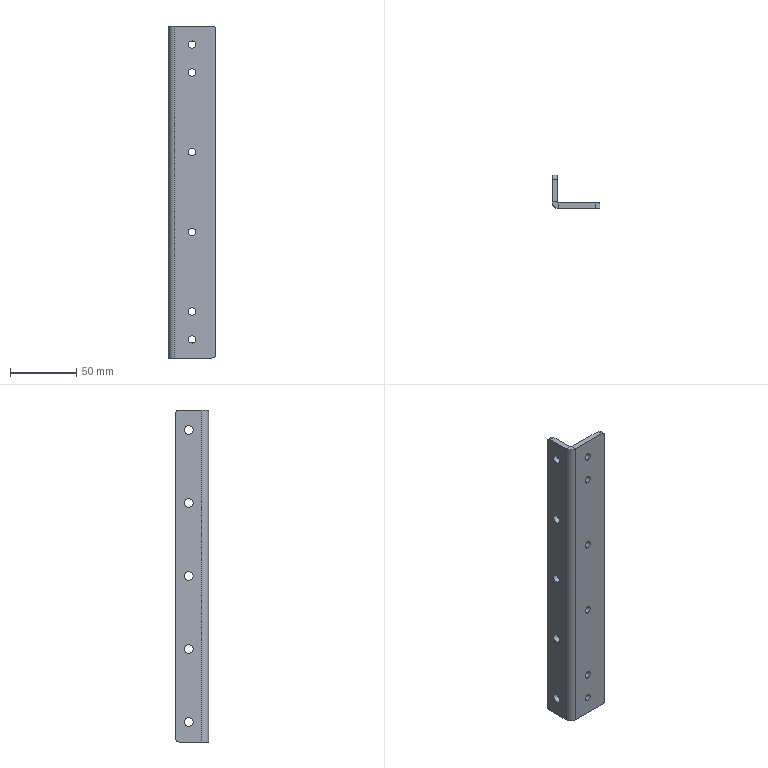Part | STEP file | Part 1 cang dai | 1 solid | 40 faces | box 36 x 25 x 250 mm | volume 54427 mm3 | cylinder 28 | plane 12 | commonest cylinder face diameters 5.5 x12 6.6 x10 6 x4 2 x1 10 x1
STEP:
#1=CARTESIAN_POINT('',(0.,15.,113.3));
#2=VERTEX_POINT('',#1);
#3=CARTESIAN_POINT('',(0.,15.,106.7));
#4=VERTEX_POINT('',#3);
#5=CARTESIAN_POINT('',(0.,15.,110.));
#6=DIRECTION('',(1.,0.,0.));
#7=DIRECTION('',(0.,0.,-1.));
#8=AXIS2_PLACEMENT_3D('',#5,#6,#7);
#9=CIRCLE('',#8,3.3);
#10=EDGE_CURVE('',#2,#4,#9,.T.);
#11=ORIENTED_EDGE('',*,*,#10,.F.);
#12=CARTESIAN_POINT('',(4.,15.,113.3));
#13=VERTEX_POINT('',#12);
#14=CARTESIAN_POINT('',(4.,15.,113.3));
#15=DIRECTION('',(1.,0.,0.));
#16=VECTOR('',#15,1000.);
#17=LINE('',#14,#16);
#18=EDGE_CURVE('',#2,#13,#17,.T.);
#19=ORIENTED_EDGE('',*,*,#18,.T.);
#20=CARTESIAN_POINT('',(4.,15.,106.7));
#21=VERTEX_POINT('',#20);
#22=CARTESIAN_POINT('',(4.,15.,110.));
#23=DIRECTION('',(1.,0.,0.));
#24=DIRECTION('',(0.,0.,-1.));
#25=AXIS2_PLACEMENT_3D('',#22,#23,#24);
#26=CIRCLE('',#25,3.3);
#27=EDGE_CURVE('',#13,#21,#26,.T.);
#28=ORIENTED_EDGE('',*,*,#27,.T.);
#29=CARTESIAN_POINT('',(4.,15.,106.7));
#30=DIRECTION('',(1.,0.,0.));
#31=VECTOR('',#30,1000.);
#32=LINE('',#29,#31);
#33=EDGE_CURVE('',#4,#21,#32,.T.);
#34=ORIENTED_EDGE('',*,*,#33,.F.);
#35=EDGE_LOOP('',(#11,#19,#28,#34));
#36=FACE_OUTER_BOUND('',#35,.T.);
#37=CARTESIAN_POINT('',(4.,15.,110.));
#38=DIRECTION('',(1.,0.,0.));
#39=DIRECTION('',(0.,0.,-1.));
#40=AXIS2_PLACEMENT_3D('',#37,#38,#39);
#41=CYLINDRICAL_SURFACE('',#40,3.3);
#42=ADVANCED_FACE('',(#36),#41,.F.);
#43=CARTESIAN_POINT('',(0.,15.,58.3));
#44=VERTEX_POINT('',#43);
#45=CARTESIAN_POINT('',(0.,15.,51.7));
#46=VERTEX_POINT('',#45);
#47=CARTESIAN_POINT('',(0.,15.,55.));
#48=DIRECTION('',(1.,0.,0.));
#49=DIRECTION('',(0.,0.,-1.));
#50=AXIS2_PLACEMENT_3D('',#47,#48,#49);
#51=CIRCLE('',#50,3.3);
#52=EDGE_CURVE('',#44,#46,#51,.T.);
#53=ORIENTED_EDGE('',*,*,#52,.F.);
#54=CARTESIAN_POINT('',(4.,15.,58.3));
#55=VERTEX_POINT('',#54);
#56=CARTESIAN_POINT('',(4.,15.,58.3));
#57=DIRECTION('',(1.,0.,0.));
#58=VECTOR('',#57,1000.);
#59=LINE('',#56,#58);
#60=EDGE_CURVE('',#44,#55,#59,.T.);
#61=ORIENTED_EDGE('',*,*,#60,.T.);
#62=CARTESIAN_POINT('',(4.,15.,51.7));
#63=VERTEX_POINT('',#62);
#64=CARTESIAN_POINT('',(4.,15.,55.));
#65=DIRECTION('',(1.,0.,0.));
#66=DIRECTION('',(0.,0.,-1.));
#67=AXIS2_PLACEMENT_3D('',#64,#65,#66);
#68=CIRCLE('',#67,3.3);
#69=EDGE_CURVE('',#55,#63,#68,.T.);
#70=ORIENTED_EDGE('',*,*,#69,.T.);
#71=CARTESIAN_POINT('',(4.,15.,51.7));
#72=DIRECTION('',(1.,0.,0.));
#73=VECTOR('',#72,1000.);
#74=LINE('',#71,#73);
#75=EDGE_CURVE('',#46,#63,#74,.T.);
#76=ORIENTED_EDGE('',*,*,#75,.F.);
#77=EDGE_LOOP('',(#53,#61,#70,#76));
#78=FACE_OUTER_BOUND('',#77,.T.);
#79=CARTESIAN_POINT('',(4.,15.,55.));
#80=DIRECTION('',(1.,0.,0.));
#81=DIRECTION('',(0.,0.,-1.));
#82=AXIS2_PLACEMENT_3D('',#79,#80,#81);
#83=CYLINDRICAL_SURFACE('',#82,3.3);
#84=ADVANCED_FACE('',(#78),#83,.F.);
#85=CARTESIAN_POINT('',(0.,15.,3.3));
#86=VERTEX_POINT('',#85);
#87=CARTESIAN_POINT('',(0.,15.,-3.3));
#88=VERTEX_POINT('',#87);
#89=CARTESIAN_POINT('',(0.,15.,0.));
#90=DIRECTION('',(1.,0.,0.));
#91=DIRECTION('',(0.,0.,-1.));
#92=AXIS2_PLACEMENT_3D('',#89,#90,#91);
#93=CIRCLE('',#92,3.3);
#94=EDGE_CURVE('',#86,#88,#93,.T.);
#95=ORIENTED_EDGE('',*,*,#94,.F.);
#96=CARTESIAN_POINT('',(4.,15.,3.3));
#97=VERTEX_POINT('',#96);
#98=CARTESIAN_POINT('',(4.,15.,3.3));
#99=DIRECTION('',(1.,0.,0.));
#100=VECTOR('',#99,1000.);
#101=LINE('',#98,#100);
#102=EDGE_CURVE('',#86,#97,#101,.T.);
#103=ORIENTED_EDGE('',*,*,#102,.T.);
#104=CARTESIAN_POINT('',(4.,15.,-3.3));
#105=VERTEX_POINT('',#104);
#106=CARTESIAN_POINT('',(4.,15.,0.));
#107=DIRECTION('',(1.,0.,0.));
#108=DIRECTION('',(0.,0.,-1.));
#109=AXIS2_PLACEMENT_3D('',#106,#107,#108);
#110=CIRCLE('',#109,3.3);
#111=EDGE_CURVE('',#97,#105,#110,.T.);
#112=ORIENTED_EDGE('',*,*,#111,.T.);
#113=CARTESIAN_POINT('',(4.,15.,-3.3));
#114=DIRECTION('',(1.,0.,0.));
#115=VECTOR('',#114,1000.);
#116=LINE('',#113,#115);
#117=EDGE_CURVE('',#88,#105,#116,.T.);
#118=ORIENTED_EDGE('',*,*,#117,.F.);
#119=EDGE_LOOP('',(#95,#103,#112,#118));
#120=FACE_OUTER_BOUND('',#119,.T.);
#121=CARTESIAN_POINT('',(4.,15.,0.));
#122=DIRECTION('',(1.,0.,0.));
#123=DIRECTION('',(0.,0.,-1.));
#124=AXIS2_PLACEMENT_3D('',#121,#122,#123);
#125=CYLINDRICAL_SURFACE('',#124,3.3);
#126=ADVANCED_FACE('',(#120),#125,.F.);
#127=CARTESIAN_POINT('',(0.,15.,-51.7));
#128=VERTEX_POINT('',#127);
#129=CARTESIAN_POINT('',(0.,15.,-58.3));
#130=VERTEX_POINT('',#129);
#131=CARTESIAN_POINT('',(0.,15.,-55.));
#132=DIRECTION('',(1.,0.,0.));
#133=DIRECTION('',(0.,0.,-1.));
#134=AXIS2_PLACEMENT_3D('',#131,#132,#133);
#135=CIRCLE('',#134,3.3);
#136=EDGE_CURVE('',#128,#130,#135,.T.);
#137=ORIENTED_EDGE('',*,*,#136,.F.);
#138=CARTESIAN_POINT('',(4.,15.,-51.7));
#139=VERTEX_POINT('',#138);
#140=CARTESIAN_POINT('',(4.,15.,-51.7));
#141=DIRECTION('',(1.,0.,0.));
#142=VECTOR('',#141,1000.);
#143=LINE('',#140,#142);
#144=EDGE_CURVE('',#128,#139,#143,.T.);
#145=ORIENTED_EDGE('',*,*,#144,.T.);
#146=CARTESIAN_POINT('',(4.,15.,-58.3));
#147=VERTEX_POINT('',#146);
#148=CARTESIAN_POINT('',(4.,15.,-55.));
#149=DIRECTION('',(1.,0.,0.));
#150=DIRECTION('',(0.,0.,-1.));
#151=AXIS2_PLACEMENT_3D('',#148,#149,#150);
#152=CIRCLE('',#151,3.3);
#153=EDGE_CURVE('',#139,#147,#152,.T.);
#154=ORIENTED_EDGE('',*,*,#153,.T.);
#155=CARTESIAN_POINT('',(4.,15.,-58.3));
#156=DIRECTION('',(1.,0.,0.));
#157=VECTOR('',#156,1000.);
#158=LINE('',#155,#157);
#159=EDGE_CURVE('',#130,#147,#158,.T.);
#160=ORIENTED_EDGE('',*,*,#159,.F.);
#161=EDGE_LOOP('',(#137,#145,#154,#160));
#162=FACE_OUTER_BOUND('',#161,.T.);
#163=CARTESIAN_POINT('',(4.,15.,-55.));
#164=DIRECTION('',(1.,0.,0.));
#165=DIRECTION('',(0.,0.,-1.));
#166=AXIS2_PLACEMENT_3D('',#163,#164,#165);
#167=CYLINDRICAL_SURFACE('',#166,3.3);
#168=ADVANCED_FACE('',(#162),#167,.F.);
#169=CARTESIAN_POINT('',(0.,15.,-106.7));
#170=VERTEX_POINT('',#169);
#171=CARTESIAN_POINT('',(0.,15.,-113.3));
#172=VERTEX_POINT('',#171);
#173=CARTESIAN_POINT('',(0.,15.,-110.));
#174=DIRECTION('',(1.,0.,0.));
#175=DIRECTION('',(0.,0.,-1.));
#176=AXIS2_PLACEMENT_3D('',#173,#174,#175);
#177=CIRCLE('',#176,3.3);
#178=EDGE_CURVE('',#170,#172,#177,.T.);
#179=ORIENTED_EDGE('',*,*,#178,.F.);
#180=CARTESIAN_POINT('',(4.,15.,-106.7));
#181=VERTEX_POINT('',#180);
#182=CARTESIAN_POINT('',(4.,15.,-106.7));
#183=DIRECTION('',(1.,0.,0.));
#184=VECTOR('',#183,1000.);
#185=LINE('',#182,#184);
#186=EDGE_CURVE('',#170,#181,#185,.T.);
#187=ORIENTED_EDGE('',*,*,#186,.T.);
#188=CARTESIAN_POINT('',(4.,15.,-113.3));
#189=VERTEX_POINT('',#188);
#190=CARTESIAN_POINT('',(4.,15.,-110.));
#191=DIRECTION('',(1.,0.,0.));
#192=DIRECTION('',(0.,0.,-1.));
#193=AXIS2_PLACEMENT_3D('',#190,#191,#192);
#194=CIRCLE('',#193,3.3);
#195=EDGE_CURVE('',#181,#189,#194,.T.);
#196=ORIENTED_EDGE('',*,*,#195,.T.);
#197=CARTESIAN_POINT('',(4.,15.,-113.3));
#198=DIRECTION('',(1.,0.,0.));
#199=VECTOR('',#198,1000.);
#200=LINE('',#197,#199);
#201=EDGE_CURVE('',#172,#189,#200,.T.);
#202=ORIENTED_EDGE('',*,*,#201,.F.);
#203=EDGE_LOOP('',(#179,#187,#196,#202));
#204=FACE_OUTER_BOUND('',#203,.T.);
#205=CARTESIAN_POINT('',(4.,15.,-110.));
#206=DIRECTION('',(1.,0.,0.));
#207=DIRECTION('',(0.,0.,-1.));
#208=AXIS2_PLACEMENT_3D('',#205,#206,#207);
#209=CYLINDRICAL_SURFACE('',#208,3.3);
#210=ADVANCED_FACE('',(#204),#209,.F.);
#211=CARTESIAN_POINT('',(18.,0.,108.25));
#212=VERTEX_POINT('',#211);
#213=CARTESIAN_POINT('',(18.,0.,113.75));
#214=VERTEX_POINT('',#213);
#215=CARTESIAN_POINT('',(18.,0.,111.));
#216=DIRECTION('',(0.,1.,0.));
#217=DIRECTION('',(0.,0.,1.));
#218=AXIS2_PLACEMENT_3D('',#215,#216,#217);
#219=CIRCLE('',#218,2.75);
#220=EDGE_CURVE('',#212,#214,#219,.T.);
#221=ORIENTED_EDGE('',*,*,#220,.F.);
#222=CARTESIAN_POINT('',(18.,4.,108.25));
#223=VERTEX_POINT('',#222);
#224=CARTESIAN_POINT('',(18.,4.,108.25));
#225=DIRECTION('',(0.,1.,0.));
#226=VECTOR('',#225,1000.);
#227=LINE('',#224,#226);
#228=EDGE_CURVE('',#212,#223,#227,.T.);
#229=ORIENTED_EDGE('',*,*,#228,.T.);
#230=CARTESIAN_POINT('',(18.,4.,113.75));
#231=VERTEX_POINT('',#230);
#232=CARTESIAN_POINT('',(18.,4.,111.));
#233=DIRECTION('',(0.,1.,0.));
#234=DIRECTION('',(0.,0.,1.));
#235=AXIS2_PLACEMENT_3D('',#232,#233,#234);
#236=CIRCLE('',#235,2.75);
#237=EDGE_CURVE('',#223,#231,#236,.T.);
#238=ORIENTED_EDGE('',*,*,#237,.T.);
#239=CARTESIAN_POINT('',(18.,4.,113.75));
#240=DIRECTION('',(0.,1.,0.));
#241=VECTOR('',#240,1000.);
#242=LINE('',#239,#241);
#243=EDGE_CURVE('',#214,#231,#242,.T.);
#244=ORIENTED_EDGE('',*,*,#243,.F.);
#245=EDGE_LOOP('',(#221,#229,#238,#244));
#246=FACE_OUTER_BOUND('',#245,.T.);
#247=CARTESIAN_POINT('',(18.,4.,111.));
#248=DIRECTION('',(0.,1.,0.));
#249=DIRECTION('',(0.,0.,1.));
#250=AXIS2_PLACEMENT_3D('',#247,#248,#249);
#251=CYLINDRICAL_SURFACE('',#250,2.75);
#252=ADVANCED_FACE('',(#246),#251,.F.);
#253=CARTESIAN_POINT('',(18.,0.,-113.75));
#254=VERTEX_POINT('',#253);
#255=CARTESIAN_POINT('',(18.,0.,-108.25));
#256=VERTEX_POINT('',#255);
#257=CARTESIAN_POINT('',(18.,0.,-111.));
#258=DIRECTION('',(0.,1.,0.));
#259=DIRECTION('',(0.,0.,1.));
#260=AXIS2_PLACEMENT_3D('',#257,#258,#259);
#261=CIRCLE('',#260,2.75);
#262=EDGE_CURVE('',#254,#256,#261,.T.);
#263=ORIENTED_EDGE('',*,*,#262,.F.);
#264=CARTESIAN_POINT('',(18.,4.,-113.75));
#265=VERTEX_POINT('',#264);
#266=CARTESIAN_POINT('',(18.,4.,-113.75));
#267=DIRECTION('',(0.,1.,0.));
#268=VECTOR('',#267,1000.);
#269=LINE('',#266,#268);
#270=EDGE_CURVE('',#254,#265,#269,.T.);
#271=ORIENTED_EDGE('',*,*,#270,.T.);
#272=CARTESIAN_POINT('',(18.,4.,-108.25));
#273=VERTEX_POINT('',#272);
#274=CARTESIAN_POINT('',(18.,4.,-111.));
#275=DIRECTION('',(0.,1.,0.));
#276=DIRECTION('',(0.,0.,1.));
#277=AXIS2_PLACEMENT_3D('',#274,#275,#276);
#278=CIRCLE('',#277,2.75);
#279=EDGE_CURVE('',#265,#273,#278,.T.);
#280=ORIENTED_EDGE('',*,*,#279,.T.);
#281=CARTESIAN_POINT('',(18.,4.,-108.25));
#282=DIRECTION('',(0.,1.,0.));
#283=VECTOR('',#282,1000.);
#284=LINE('',#281,#283);
#285=EDGE_CURVE('',#256,#273,#284,.T.);
#286=ORIENTED_EDGE('',*,*,#285,.F.);
#287=EDGE_LOOP('',(#263,#271,#280,#286));
#288=FACE_OUTER_BOUND('',#287,.T.);
#289=CARTESIAN_POINT('',(18.,4.,-111.));
#290=DIRECTION('',(0.,1.,0.));
#291=DIRECTION('',(0.,0.,1.));
#292=AXIS2_PLACEMENT_3D('',#289,#290,#291);
#293=CYLINDRICAL_SURFACE('',#292,2.75);
#294=ADVANCED_FACE('',(#288),#293,.F.);
#295=CARTESIAN_POINT('',(18.,0.,-92.75));
#296=VERTEX_POINT('',#295);
#297=CARTESIAN_POINT('',(18.,0.,-87.25));
#298=VERTEX_POINT('',#297);
#299=CARTESIAN_POINT('',(18.,0.,-90.));
#300=DIRECTION('',(0.,1.,0.));
#301=DIRECTION('',(0.,0.,1.));
#302=AXIS2_PLACEMENT_3D('',#299,#300,#301);
#303=CIRCLE('',#302,2.75);
#304=EDGE_CURVE('',#296,#298,#303,.T.);
#305=ORIENTED_EDGE('',*,*,#304,.F.);
#306=CARTESIAN_POINT('',(18.,4.,-92.75));
#307=VERTEX_POINT('',#306);
#308=CARTESIAN_POINT('',(18.,4.,-92.75));
#309=DIRECTION('',(0.,1.,0.));
#310=VECTOR('',#309,1000.);
#311=LINE('',#308,#310);
#312=EDGE_CURVE('',#296,#307,#311,.T.);
#313=ORIENTED_EDGE('',*,*,#312,.T.);
#314=CARTESIAN_POINT('',(18.,4.,-87.25));
#315=VERTEX_POINT('',#314);
#316=CARTESIAN_POINT('',(18.,4.,-90.));
#317=DIRECTION('',(0.,1.,0.));
#318=DIRECTION('',(0.,0.,1.));
#319=AXIS2_PLACEMENT_3D('',#316,#317,#318);
#320=CIRCLE('',#319,2.75);
#321=EDGE_CURVE('',#307,#315,#320,.T.);
#322=ORIENTED_EDGE('',*,*,#321,.T.);
#323=CARTESIAN_POINT('',(18.,4.,-87.25));
#324=DIRECTION('',(0.,1.,0.));
#325=VECTOR('',#324,1000.);
#326=LINE('',#323,#325);
#327=EDGE_CURVE('',#298,#315,#326,.T.);
#328=ORIENTED_EDGE('',*,*,#327,.F.);
#329=EDGE_LOOP('',(#305,#313,#322,#328));
#330=FACE_OUTER_BOUND('',#329,.T.);
#331=CARTESIAN_POINT('',(18.,4.,-90.));
#332=DIRECTION('',(0.,1.,0.));
#333=DIRECTION('',(0.,0.,1.));
#334=AXIS2_PLACEMENT_3D('',#331,#332,#333);
#335=CYLINDRICAL_SURFACE('',#334,2.75);
#336=ADVANCED_FACE('',(#330),#335,.F.);
#337=CARTESIAN_POINT('',(18.,0.,-32.75));
#338=VERTEX_POINT('',#337);
#339=CARTESIAN_POINT('',(18.,0.,-27.25));
#340=VERTEX_POINT('',#339);
#341=CARTESIAN_POINT('',(18.,0.,-30.));
#342=DIRECTION('',(0.,1.,0.));
#343=DIRECTION('',(0.,0.,1.));
#344=AXIS2_PLACEMENT_3D('',#341,#342,#343);
#345=CIRCLE('',#344,2.75);
#346=EDGE_CURVE('',#338,#340,#345,.T.);
#347=ORIENTED_EDGE('',*,*,#346,.F.);
#348=CARTESIAN_POINT('',(18.,4.,-32.75));
#349=VERTEX_POINT('',#348);
#350=CARTESIAN_POINT('',(18.,4.,-32.75));
#351=DIRECTION('',(0.,1.,0.));
#352=VECTOR('',#351,1000.);
#353=LINE('',#350,#352);
#354=EDGE_CURVE('',#338,#349,#353,.T.);
#355=ORIENTED_EDGE('',*,*,#354,.T.);
#356=CARTESIAN_POINT('',(18.,4.,-27.25));
#357=VERTEX_POINT('',#356);
#358=CARTESIAN_POINT('',(18.,4.,-30.));
#359=DIRECTION('',(0.,1.,0.));
#360=DIRECTION('',(0.,0.,1.));
#361=AXIS2_PLACEMENT_3D('',#358,#359,#360);
#362=CIRCLE('',#361,2.75);
#363=EDGE_CURVE('',#349,#357,#362,.T.);
#364=ORIENTED_EDGE('',*,*,#363,.T.);
#365=CARTESIAN_POINT('',(18.,4.,-27.25));
#366=DIRECTION('',(0.,1.,0.));
#367=VECTOR('',#366,1000.);
#368=LINE('',#365,#367);
#369=EDGE_CURVE('',#340,#357,#368,.T.);
#370=ORIENTED_EDGE('',*,*,#369,.F.);
#371=EDGE_LOOP('',(#347,#355,#364,#370));
#372=FACE_OUTER_BOUND('',#371,.T.);
#373=CARTESIAN_POINT('',(18.,4.,-30.));
#374=DIRECTION('',(0.,1.,0.));
#375=DIRECTION('',(0.,0.,1.));
#376=AXIS2_PLACEMENT_3D('',#373,#374,#375);
#377=CYLINDRICAL_SURFACE('',#376,2.75);
#378=ADVANCED_FACE('',(#372),#377,.F.);
#379=CARTESIAN_POINT('',(18.,0.,27.25));
#380=VERTEX_POINT('',#379);
#381=CARTESIAN_POINT('',(18.,0.,32.75));
#382=VERTEX_POINT('',#381);
#383=CARTESIAN_POINT('',(18.,0.,30.));
#384=DIRECTION('',(0.,1.,0.));
#385=DIRECTION('',(0.,0.,1.));
#386=AXIS2_PLACEMENT_3D('',#383,#384,#385);
#387=CIRCLE('',#386,2.75);
#388=EDGE_CURVE('',#380,#382,#387,.T.);
#389=ORIENTED_EDGE('',*,*,#388,.F.);
#390=CARTESIAN_POINT('',(18.,4.,27.25));
#391=VERTEX_POINT('',#390);
#392=CARTESIAN_POINT('',(18.,4.,27.25));
#393=DIRECTION('',(0.,1.,0.));
#394=VECTOR('',#393,1000.);
#395=LINE('',#392,#394);
#396=EDGE_CURVE('',#380,#391,#395,.T.);
#397=ORIENTED_EDGE('',*,*,#396,.T.);
#398=CARTESIAN_POINT('',(18.,4.,32.75));
#399=VERTEX_POINT('',#398);
#400=CARTESIAN_POINT('',(18.,4.,30.));
#401=DIRECTION('',(0.,1.,0.));
#402=DIRECTION('',(0.,0.,1.));
#403=AXIS2_PLACEMENT_3D('',#400,#401,#402);
#404=CIRCLE('',#403,2.75);
#405=EDGE_CURVE('',#391,#399,#404,.T.);
#406=ORIENTED_EDGE('',*,*,#405,.T.);
#407=CARTESIAN_POINT('',(18.,4.,32.75));
#408=DIRECTION('',(0.,1.,0.));
#409=VECTOR('',#408,1000.);
#410=LINE('',#407,#409);
#411=EDGE_CURVE('',#382,#399,#410,.T.);
#412=ORIENTED_EDGE('',*,*,#411,.F.);
#413=EDGE_LOOP('',(#389,#397,#406,#412));
#414=FACE_OUTER_BOUND('',#413,.T.);
#415=CARTESIAN_POINT('',(18.,4.,30.));
#416=DIRECTION('',(0.,1.,0.));
#417=DIRECTION('',(0.,0.,1.));
#418=AXIS2_PLACEMENT_3D('',#415,#416,#417);
#419=CYLINDRICAL_SURFACE('',#418,2.75);
#420=ADVANCED_FACE('',(#414),#419,.F.);
#421=CARTESIAN_POINT('',(18.,0.,87.25));
#422=VERTEX_POINT('',#421);
#423=CARTESIAN_POINT('',(18.,0.,92.75));
#424=VERTEX_POINT('',#423);
#425=CARTESIAN_POINT('',(18.,0.,90.));
#426=DIRECTION('',(0.,1.,0.));
#427=DIRECTION('',(0.,0.,1.));
#428=AXIS2_PLACEMENT_3D('',#425,#426,#427);
#429=CIRCLE('',#428,2.75);
#430=EDGE_CURVE('',#422,#424,#429,.T.);
#431=ORIENTED_EDGE('',*,*,#430,.F.);
#432=CARTESIAN_POINT('',(18.,4.,87.25));
#433=VERTEX_POINT('',#432);
#434=CARTESIAN_POINT('',(18.,4.,87.25));
#435=DIRECTION('',(0.,1.,0.));
#436=VECTOR('',#435,1000.);
#437=LINE('',#434,#436);
#438=EDGE_CURVE('',#422,#433,#437,.T.);
#439=ORIENTED_EDGE('',*,*,#438,.T.);
#440=CARTESIAN_POINT('',(18.,4.,92.75));
#441=VERTEX_POINT('',#440);
#442=CARTESIAN_POINT('',(18.,4.,90.));
#443=DIRECTION('',(0.,1.,0.));
#444=DIRECTION('',(0.,0.,1.));
#445=AXIS2_PLACEMENT_3D('',#442,#443,#444);
#446=CIRCLE('',#445,2.75);
#447=EDGE_CURVE('',#433,#441,#446,.T.);
#448=ORIENTED_EDGE('',*,*,#447,.T.);
#449=CARTESIAN_POINT('',(18.,4.,92.75));
#450=DIRECTION('',(0.,1.,0.));
#451=VECTOR('',#450,1000.);
#452=LINE('',#449,#451);
#453=EDGE_CURVE('',#424,#441,#452,.T.);
#454=ORIENTED_EDGE('',*,*,#453,.F.);
#455=EDGE_LOOP('',(#431,#439,#448,#454));
#456=FACE_OUTER_BOUND('',#455,.T.);
#457=CARTESIAN_POINT('',(18.,4.,90.));
#458=DIRECTION('',(0.,1.,0.));
#459=DIRECTION('',(0.,0.,1.));
#460=AXIS2_PLACEMENT_3D('',#457,#458,#459);
#461=CYLINDRICAL_SURFACE('',#460,2.75);
#462=ADVANCED_FACE('',(#456),#461,.F.);
#463=CARTESIAN_POINT('',(0.,5.,125.));
#464=VERTEX_POINT('',#463);
#465=CARTESIAN_POINT('',(4.,5.,125.));
#466=VERTEX_POINT('',#465);
#467=CARTESIAN_POINT('',(0.,5.,125.));
#468=DIRECTION('',(1.,0.,0.));
#469=VECTOR('',#468,1000.);
#470=LINE('',#467,#469);
#471=EDGE_CURVE('',#464,#466,#470,.T.);
#472=ORIENTED_EDGE('',*,*,#471,.F.);
#473=CARTESIAN_POINT('',(5.,0.,125.));
#474=VERTEX_POINT('',#473);
#475=CARTESIAN_POINT('',(5.,5.,125.));
#476=DIRECTION('',(0.,0.,1.));
#477=DIRECTION('',(-1.,0.,0.));
#478=AXIS2_PLACEMENT_3D('',#475,#476,#477);
#479=CIRCLE('',#478,5.);
#480=EDGE_CURVE('',#464,#474,#479,.T.);
#481=ORIENTED_EDGE('',*,*,#480,.T.);
#482=CARTESIAN_POINT('',(5.,4.,125.));
#483=VERTEX_POINT('',#482);
#484=CARTESIAN_POINT('',(5.,4.,125.));
#485=DIRECTION('',(0.,-1.,0.));
#486=VECTOR('',#485,1000.);
#487=LINE('',#484,#486);
#488=EDGE_CURVE('',#483,#474,#487,.T.);
#489=ORIENTED_EDGE('',*,*,#488,.F.);
#490=CARTESIAN_POINT('',(5.,5.,125.));
#491=DIRECTION('',(0.,0.,1.));
#492=DIRECTION('',(1.,0.,0.));
#493=AXIS2_PLACEMENT_3D('',#490,#491,#492);
#494=CIRCLE('',#493,1.);
#495=EDGE_CURVE('',#466,#483,#494,.T.);
#496=ORIENTED_EDGE('',*,*,#495,.F.);
#497=EDGE_LOOP('',(#472,#481,#489,#496));
#498=FACE_OUTER_BOUND('',#497,.T.);
#499=CARTESIAN_POINT('',(0.,5.,125.));
#500=DIRECTION('',(0.,0.,1.));
#501=DIRECTION('',(1.,0.,0.));
#502=AXIS2_PLACEMENT_3D('',#499,#500,#501);
#503=PLANE('',#502);
#504=ADVANCED_FACE('',(#498),#503,.T.);
#505=CARTESIAN_POINT('',(4.,22.,125.));
#506=VERTEX_POINT('',#505);
#507=CARTESIAN_POINT('',(4.,0.,125.));
#508=DIRECTION('',(0.,-1.,0.));
#509=VECTOR('',#508,1000.);
#510=LINE('',#507,#509);
#511=EDGE_CURVE('',#506,#466,#510,.T.);
#512=ORIENTED_EDGE('',*,*,#511,.F.);
#513=CARTESIAN_POINT('',(0.,22.,125.));
#514=VERTEX_POINT('',#513);
#515=CARTESIAN_POINT('',(5.,22.,125.));
#516=DIRECTION('',(-1.,0.,0.));
#517=VECTOR('',#516,1000.);
#518=LINE('',#515,#517);
#519=EDGE_CURVE('',#506,#514,#518,.T.);
#520=ORIENTED_EDGE('',*,*,#519,.T.);
#521=CARTESIAN_POINT('',(0.,0.,125.));
#522=DIRECTION('',(0.,-1.,0.));
#523=VECTOR('',#522,1000.);
#524=LINE('',#521,#523);
#525=EDGE_CURVE('',#514,#464,#524,.T.);
#526=ORIENTED_EDGE('',*,*,#525,.T.);
#527=ORIENTED_EDGE('',*,*,#471,.T.);
#528=EDGE_LOOP('',(#512,#520,#526,#527));
#529=FACE_OUTER_BOUND('',#528,.T.);
#530=CARTESIAN_POINT('',(5.,4.,125.));
#531=DIRECTION('',(0.,0.,1.));
#532=DIRECTION('',(1.,0.,0.));
#533=AXIS2_PLACEMENT_3D('',#530,#531,#532);
#534=PLANE('',#533);
#535=ADVANCED_FACE('',(#529),#534,.T.);
#536=CARTESIAN_POINT('',(5.,0.,-125.));
#537=VERTEX_POINT('',#536);
#538=CARTESIAN_POINT('',(5.,4.,-125.));
#539=VERTEX_POINT('',#538);
#540=CARTESIAN_POINT('',(5.,0.,-125.));
#541=DIRECTION('',(0.,1.,0.));
#542=VECTOR('',#541,1000.);
#543=LINE('',#540,#542);
#544=EDGE_CURVE('',#537,#539,#543,.T.);
#545=ORIENTED_EDGE('',*,*,#544,.F.);
#546=CARTESIAN_POINT('',(0.,5.,-125.));
#547=VERTEX_POINT('',#546);
#548=CARTESIAN_POINT('',(5.,5.,-125.));
#549=DIRECTION('',(0.,0.,1.));
#550=DIRECTION('',(-1.,0.,0.));
#551=AXIS2_PLACEMENT_3D('',#548,#549,#550);
#552=CIRCLE('',#551,5.);
#553=EDGE_CURVE('',#547,#537,#552,.T.);
#554=ORIENTED_EDGE('',*,*,#553,.F.);
#555=CARTESIAN_POINT('',(4.,5.,-125.));
#556=VERTEX_POINT('',#555);
#557=CARTESIAN_POINT('',(4.,5.,-125.));
#558=DIRECTION('',(-1.,0.,0.));
#559=VECTOR('',#558,1000.);
#560=LINE('',#557,#559);
#561=EDGE_CURVE('',#556,#547,#560,.T.);
#562=ORIENTED_EDGE('',*,*,#561,.F.);
#563=CARTESIAN_POINT('',(5.,5.,-125.));
#564=DIRECTION('',(0.,0.,1.));
#565=DIRECTION('',(1.,0.,0.));
#566=AXIS2_PLACEMENT_3D('',#563,#564,#565);
#567=CIRCLE('',#566,1.);
#568=EDGE_CURVE('',#556,#539,#567,.T.);
#569=ORIENTED_EDGE('',*,*,#568,.T.);
#570=EDGE_LOOP('',(#545,#554,#562,#569));
#571=FACE_OUTER_BOUND('',#570,.T.);
#572=CARTESIAN_POINT('',(5.,0.,-125.));
#573=DIRECTION('',(0.,0.,-1.));
#574=DIRECTION('',(-1.,0.,0.));
#575=AXIS2_PLACEMENT_3D('',#572,#573,#574);
#576=PLANE('',#575);
#577=ADVANCED_FACE('',(#571),#576,.T.);
#578=CARTESIAN_POINT('',(33.,4.,-125.));
#579=VERTEX_POINT('',#578);
#580=CARTESIAN_POINT('',(0.,4.,-125.));
#581=DIRECTION('',(1.,0.,0.));
#582=VECTOR('',#581,1000.);
#583=LINE('',#580,#582);
#584=EDGE_CURVE('',#539,#579,#583,.T.);
#585=ORIENTED_EDGE('',*,*,#584,.T.);
#586=CARTESIAN_POINT('',(33.,0.,-125.));
#587=VERTEX_POINT('',#586);
#588=CARTESIAN_POINT('',(33.,5.,-125.));
#589=DIRECTION('',(0.,-1.,0.));
#590=VECTOR('',#589,1000.);
#591=LINE('',#588,#590);
#592=EDGE_CURVE('',#579,#587,#591,.T.);
#593=ORIENTED_EDGE('',*,*,#592,.T.);
#594=CARTESIAN_POINT('',(0.,0.,-125.));
#595=DIRECTION('',(1.,0.,0.));
#596=VECTOR('',#595,1000.);
#597=LINE('',#594,#596);
#598=EDGE_CURVE('',#537,#587,#597,.T.);
#599=ORIENTED_EDGE('',*,*,#598,.F.);
#600=ORIENTED_EDGE('',*,*,#544,.T.);
#601=EDGE_LOOP('',(#585,#593,#599,#600));
#602=FACE_OUTER_BOUND('',#601,.T.);
#603=CARTESIAN_POINT('',(4.,5.,-125.));
#604=DIRECTION('',(0.,0.,-1.));
#605=DIRECTION('',(-1.,0.,0.));
#606=AXIS2_PLACEMENT_3D('',#603,#604,#605);
#607=PLANE('',#606);
#608=ADVANCED_FACE('',(#602),#607,.T.);
#609=CARTESIAN_POINT('',(18.,0.,111.));
#610=DIRECTION('',(0.,1.,0.));
#611=DIRECTION('',(0.,0.,1.));
#612=AXIS2_PLACEMENT_3D('',#609,#610,#611);
#613=CIRCLE('',#612,2.75);
#614=EDGE_CURVE('',#214,#212,#613,.T.);
#615=ORIENTED_EDGE('',*,*,#614,.T.);
#616=ORIENTED_EDGE('',*,*,#220,.T.);
#617=EDGE_LOOP('',(#615,#616));
#618=FACE_BOUND('',#617,.T.);
#619=CARTESIAN_POINT('',(18.,0.,-111.));
#620=DIRECTION('',(0.,1.,0.));
#621=DIRECTION('',(0.,0.,1.));
#622=AXIS2_PLACEMENT_3D('',#619,#620,#621);
#623=CIRCLE('',#622,2.75);
#624=EDGE_CURVE('',#256,#254,#623,.T.);
#625=ORIENTED_EDGE('',*,*,#624,.T.);
#626=ORIENTED_EDGE('',*,*,#262,.T.);
#627=EDGE_LOOP('',(#625,#626));
#628=FACE_BOUND('',#627,.T.);
#629=CARTESIAN_POINT('',(18.,0.,-90.));
#630=DIRECTION('',(0.,1.,0.));
#631=DIRECTION('',(0.,0.,1.));
#632=AXIS2_PLACEMENT_3D('',#629,#630,#631);
#633=CIRCLE('',#632,2.75);
#634=EDGE_CURVE('',#298,#296,#633,.T.);
#635=ORIENTED_EDGE('',*,*,#634,.T.);
#636=ORIENTED_EDGE('',*,*,#304,.T.);
#637=EDGE_LOOP('',(#635,#636));
#638=FACE_BOUND('',#637,.T.);
#639=CARTESIAN_POINT('',(18.,0.,-30.));
#640=DIRECTION('',(0.,1.,0.));
#641=DIRECTION('',(0.,0.,1.));
#642=AXIS2_PLACEMENT_3D('',#639,#640,#641);
#643=CIRCLE('',#642,2.75);
#644=EDGE_CURVE('',#340,#338,#643,.T.);
#645=ORIENTED_EDGE('',*,*,#644,.T.);
#646=ORIENTED_EDGE('',*,*,#346,.T.);
#647=EDGE_LOOP('',(#645,#646));
#648=FACE_BOUND('',#647,.T.);
#649=CARTESIAN_POINT('',(18.,0.,30.));
#650=DIRECTION('',(0.,1.,0.));
#651=DIRECTION('',(0.,0.,1.));
#652=AXIS2_PLACEMENT_3D('',#649,#650,#651);
#653=CIRCLE('',#652,2.75);
#654=EDGE_CURVE('',#382,#380,#653,.T.);
#655=ORIENTED_EDGE('',*,*,#654,.T.);
#656=ORIENTED_EDGE('',*,*,#388,.T.);
#657=EDGE_LOOP('',(#655,#656));
#658=FACE_BOUND('',#657,.T.);
#659=CARTESIAN_POINT('',(18.,0.,90.));
#660=DIRECTION('',(0.,1.,0.));
#661=DIRECTION('',(0.,0.,1.));
#662=AXIS2_PLACEMENT_3D('',#659,#660,#661);
#663=CIRCLE('',#662,2.75);
#664=EDGE_CURVE('',#424,#422,#663,.T.);
#665=ORIENTED_EDGE('',*,*,#664,.T.);
#666=ORIENTED_EDGE('',*,*,#430,.T.);
#667=EDGE_LOOP('',(#665,#666));
#668=FACE_BOUND('',#667,.T.);
#669=ORIENTED_EDGE('',*,*,#598,.T.);
#670=CARTESIAN_POINT('',(36.,0.,-122.));
#671=VERTEX_POINT('',#670);
#672=CARTESIAN_POINT('',(33.,0.,-122.));
#673=DIRECTION('',(0.,-1.,0.));
#674=DIRECTION('',(0.,0.,1.));
#675=AXIS2_PLACEMENT_3D('',#672,#673,#674);
#676=CIRCLE('',#675,3.);
#677=EDGE_CURVE('',#587,#671,#676,.T.);
#678=ORIENTED_EDGE('',*,*,#677,.T.);
#679=CARTESIAN_POINT('',(36.,0.,122.));
#680=VERTEX_POINT('',#679);
#681=CARTESIAN_POINT('',(36.,0.,125.));
#682=DIRECTION('',(0.,0.,-1.));
#683=VECTOR('',#682,1000.);
#684=LINE('',#681,#683);
#685=EDGE_CURVE('',#680,#671,#684,.T.);
#686=ORIENTED_EDGE('',*,*,#685,.F.);
#687=CARTESIAN_POINT('',(33.,0.,125.));
#688=VERTEX_POINT('',#687);
#689=CARTESIAN_POINT('',(33.,0.,122.));
#690=DIRECTION('',(0.,-1.,0.));
#691=DIRECTION('',(0.,0.,1.));
#692=AXIS2_PLACEMENT_3D('',#689,#690,#691);
#693=CIRCLE('',#692,3.);
#694=EDGE_CURVE('',#680,#688,#693,.T.);
#695=ORIENTED_EDGE('',*,*,#694,.T.);
#696=CARTESIAN_POINT('',(0.,0.,125.));
#697=DIRECTION('',(1.,0.,0.));
#698=VECTOR('',#697,1000.);
#699=LINE('',#696,#698);
#700=EDGE_CURVE('',#474,#688,#699,.T.);
#701=ORIENTED_EDGE('',*,*,#700,.F.);
#702=CARTESIAN_POINT('',(5.,0.,125.));
#703=DIRECTION('',(0.,0.,-1.));
#704=VECTOR('',#703,1000.);
#705=LINE('',#702,#704);
#706=EDGE_CURVE('',#474,#537,#705,.T.);
#707=ORIENTED_EDGE('',*,*,#706,.T.);
#708=EDGE_LOOP('',(#669,#678,#686,#695,#701,#707));
#709=FACE_OUTER_BOUND('',#708,.T.);
#710=CARTESIAN_POINT('',(0.,0.,125.));
#711=DIRECTION('',(0.,1.,0.));
#712=DIRECTION('',(0.,0.,1.));
#713=AXIS2_PLACEMENT_3D('',#710,#711,#712);
#714=PLANE('',#713);
#715=ADVANCED_FACE('',(#618,#628,#638,#648,#658,#668,#709),#714,.F.);
#716=ORIENTED_EDGE('',*,*,#685,.T.);
#717=CARTESIAN_POINT('',(36.,4.,-122.));
#718=VERTEX_POINT('',#717);
#719=CARTESIAN_POINT('',(36.,4.,-122.));
#720=DIRECTION('',(0.,1.,0.));
#721=VECTOR('',#720,1000.);
#722=LINE('',#719,#721);
#723=EDGE_CURVE('',#671,#718,#722,.T.);
#724=ORIENTED_EDGE('',*,*,#723,.T.);
#725=CARTESIAN_POINT('',(36.,4.,122.));
#726=VERTEX_POINT('',#725);
#727=CARTESIAN_POINT('',(36.,4.,125.));
#728=DIRECTION('',(0.,0.,-1.));
#729=VECTOR('',#728,1000.);
#730=LINE('',#727,#729);
#731=EDGE_CURVE('',#726,#718,#730,.T.);
#732=ORIENTED_EDGE('',*,*,#731,.F.);
#733=CARTESIAN_POINT('',(36.,4.,122.));
#734=DIRECTION('',(0.,-1.,0.));
#735=VECTOR('',#734,1000.);
#736=LINE('',#733,#735);
#737=EDGE_CURVE('',#726,#680,#736,.T.);
#738=ORIENTED_EDGE('',*,*,#737,.T.);
#739=EDGE_LOOP('',(#716,#724,#732,#738));
#740=FACE_OUTER_BOUND('',#739,.T.);
#741=CARTESIAN_POINT('',(36.,4.,125.));
#742=DIRECTION('',(1.,0.,0.));
#743=DIRECTION('',(0.,0.,-1.));
#744=AXIS2_PLACEMENT_3D('',#741,#742,#743);
#745=PLANE('',#744);
#746=ADVANCED_FACE('',(#740),#745,.T.);
#747=CARTESIAN_POINT('',(18.,4.,111.));
#748=DIRECTION('',(0.,1.,0.));
#749=DIRECTION('',(0.,0.,1.));
#750=AXIS2_PLACEMENT_3D('',#747,#748,#749);
#751=CIRCLE('',#750,2.75);
#752=EDGE_CURVE('',#231,#223,#751,.T.);
#753=ORIENTED_EDGE('',*,*,#752,.F.);
#754=ORIENTED_EDGE('',*,*,#237,.F.);
#755=EDGE_LOOP('',(#753,#754));
#756=FACE_BOUND('',#755,.T.);
#757=CARTESIAN_POINT('',(18.,4.,-111.));
#758=DIRECTION('',(0.,1.,0.));
#759=DIRECTION('',(0.,0.,1.));
#760=AXIS2_PLACEMENT_3D('',#757,#758,#759);
#761=CIRCLE('',#760,2.75);
#762=EDGE_CURVE('',#273,#265,#761,.T.);
#763=ORIENTED_EDGE('',*,*,#762,.F.);
#764=ORIENTED_EDGE('',*,*,#279,.F.);
#765=EDGE_LOOP('',(#763,#764));
#766=FACE_BOUND('',#765,.T.);
#767=CARTESIAN_POINT('',(18.,4.,-90.));
#768=DIRECTION('',(0.,1.,0.));
#769=DIRECTION('',(0.,0.,1.));
#770=AXIS2_PLACEMENT_3D('',#767,#768,#769);
#771=CIRCLE('',#770,2.75);
#772=EDGE_CURVE('',#315,#307,#771,.T.);
#773=ORIENTED_EDGE('',*,*,#772,.F.);
#774=ORIENTED_EDGE('',*,*,#321,.F.);
#775=EDGE_LOOP('',(#773,#774));
#776=FACE_BOUND('',#775,.T.);
#777=CARTESIAN_POINT('',(18.,4.,-30.));
#778=DIRECTION('',(0.,1.,0.));
#779=DIRECTION('',(0.,0.,1.));
#780=AXIS2_PLACEMENT_3D('',#777,#778,#779);
#781=CIRCLE('',#780,2.75);
#782=EDGE_CURVE('',#357,#349,#781,.T.);
#783=ORIENTED_EDGE('',*,*,#782,.F.);
#784=ORIENTED_EDGE('',*,*,#363,.F.);
#785=EDGE_LOOP('',(#783,#784));
#786=FACE_BOUND('',#785,.T.);
#787=CARTESIAN_POINT('',(18.,4.,30.));
#788=DIRECTION('',(0.,1.,0.));
#789=DIRECTION('',(0.,0.,1.));
#790=AXIS2_PLACEMENT_3D('',#787,#788,#789);
#791=CIRCLE('',#790,2.75);
#792=EDGE_CURVE('',#399,#391,#791,.T.);
#793=ORIENTED_EDGE('',*,*,#792,.F.);
#794=ORIENTED_EDGE('',*,*,#405,.F.);
#795=EDGE_LOOP('',(#793,#794));
#796=FACE_BOUND('',#795,.T.);
#797=CARTESIAN_POINT('',(18.,4.,90.));
#798=DIRECTION('',(0.,1.,0.));
#799=DIRECTION('',(0.,0.,1.));
#800=AXIS2_PLACEMENT_3D('',#797,#798,#799);
#801=CIRCLE('',#800,2.75);
#802=EDGE_CURVE('',#441,#433,#801,.T.);
#803=ORIENTED_EDGE('',*,*,#802,.F.);
#804=ORIENTED_EDGE('',*,*,#447,.F.);
#805=EDGE_LOOP('',(#803,#804));
#806=FACE_BOUND('',#805,.T.);
#807=ORIENTED_EDGE('',*,*,#731,.T.);
#808=CARTESIAN_POINT('',(33.,4.,-122.));
#809=DIRECTION('',(0.,1.,0.));
#810=DIRECTION('',(0.,0.,1.));
#811=AXIS2_PLACEMENT_3D('',#808,#809,#810);
#812=CIRCLE('',#811,3.);
#813=EDGE_CURVE('',#718,#579,#812,.T.);
#814=ORIENTED_EDGE('',*,*,#813,.T.);
#815=ORIENTED_EDGE('',*,*,#584,.F.);
#816=CARTESIAN_POINT('',(5.,4.,125.));
#817=DIRECTION('',(0.,0.,-1.));
#818=VECTOR('',#817,1000.);
#819=LINE('',#816,#818);
#820=EDGE_CURVE('',#483,#539,#819,.T.);
#821=ORIENTED_EDGE('',*,*,#820,.F.);
#822=CARTESIAN_POINT('',(33.,4.,125.));
#823=VERTEX_POINT('',#822);
#824=CARTESIAN_POINT('',(0.,4.,125.));
#825=DIRECTION('',(1.,0.,0.));
#826=VECTOR('',#825,1000.);
#827=LINE('',#824,#826);
#828=EDGE_CURVE('',#483,#823,#827,.T.);
#829=ORIENTED_EDGE('',*,*,#828,.T.);
#830=CARTESIAN_POINT('',(33.,4.,122.));
#831=DIRECTION('',(0.,1.,0.));
#832=DIRECTION('',(0.,0.,1.));
#833=AXIS2_PLACEMENT_3D('',#830,#831,#832);
#834=CIRCLE('',#833,3.);
#835=EDGE_CURVE('',#823,#726,#834,.T.);
#836=ORIENTED_EDGE('',*,*,#835,.T.);
#837=EDGE_LOOP('',(#807,#814,#815,#821,#829,#836));
#838=FACE_OUTER_BOUND('',#837,.T.);
#839=CARTESIAN_POINT('',(0.,4.,125.));
#840=DIRECTION('',(0.,1.,0.));
#841=DIRECTION('',(0.,0.,1.));
#842=AXIS2_PLACEMENT_3D('',#839,#840,#841);
#843=PLANE('',#842);
#844=ADVANCED_FACE('',(#756,#766,#776,#786,#796,#806,#838),#843,.T.);
#845=ORIENTED_EDGE('',*,*,#568,.F.);
#846=CARTESIAN_POINT('',(4.,5.,125.));
#847=DIRECTION('',(0.,0.,-1.));
#848=VECTOR('',#847,1000.);
#849=LINE('',#846,#848);
#850=EDGE_CURVE('',#466,#556,#849,.T.);
#851=ORIENTED_EDGE('',*,*,#850,.F.);
#852=ORIENTED_EDGE('',*,*,#495,.T.);
#853=ORIENTED_EDGE('',*,*,#820,.T.);
#854=EDGE_LOOP('',(#845,#851,#852,#853));
#855=FACE_OUTER_BOUND('',#854,.T.);
#856=CARTESIAN_POINT('',(5.,5.,125.));
#857=DIRECTION('',(0.,0.,-1.));
#858=DIRECTION('',(-1.,0.,0.));
#859=AXIS2_PLACEMENT_3D('',#856,#857,#858);
#860=CYLINDRICAL_SURFACE('',#859,1.);
#861=ADVANCED_FACE('',(#855),#860,.F.);
#862=CARTESIAN_POINT('',(4.,15.,110.));
#863=DIRECTION('',(1.,0.,0.));
#864=DIRECTION('',(0.,0.,-1.));
#865=AXIS2_PLACEMENT_3D('',#862,#863,#864);
#866=CIRCLE('',#865,3.3);
#867=EDGE_CURVE('',#21,#13,#866,.T.);
#868=ORIENTED_EDGE('',*,*,#867,.F.);
#869=ORIENTED_EDGE('',*,*,#27,.F.);
#870=EDGE_LOOP('',(#868,#869));
#871=FACE_BOUND('',#870,.T.);
#872=CARTESIAN_POINT('',(4.,15.,55.));
#873=DIRECTION('',(1.,0.,0.));
#874=DIRECTION('',(0.,0.,-1.));
#875=AXIS2_PLACEMENT_3D('',#872,#873,#874);
#876=CIRCLE('',#875,3.3);
#877=EDGE_CURVE('',#63,#55,#876,.T.);
#878=ORIENTED_EDGE('',*,*,#877,.F.);
#879=ORIENTED_EDGE('',*,*,#69,.F.);
#880=EDGE_LOOP('',(#878,#879));
#881=FACE_BOUND('',#880,.T.);
#882=CARTESIAN_POINT('',(4.,15.,0.));
#883=DIRECTION('',(1.,0.,0.));
#884=DIRECTION('',(0.,0.,-1.));
#885=AXIS2_PLACEMENT_3D('',#882,#883,#884);
#886=CIRCLE('',#885,3.3);
#887=EDGE_CURVE('',#105,#97,#886,.T.);
#888=ORIENTED_EDGE('',*,*,#887,.F.);
#889=ORIENTED_EDGE('',*,*,#111,.F.);
#890=EDGE_LOOP('',(#888,#889));
#891=FACE_BOUND('',#890,.T.);
#892=CARTESIAN_POINT('',(4.,15.,-55.));
#893=DIRECTION('',(1.,0.,0.));
#894=DIRECTION('',(0.,0.,-1.));
#895=AXIS2_PLACEMENT_3D('',#892,#893,#894);
#896=CIRCLE('',#895,3.3);
#897=EDGE_CURVE('',#147,#139,#896,.T.);
#898=ORIENTED_EDGE('',*,*,#897,.F.);
#899=ORIENTED_EDGE('',*,*,#153,.F.);
#900=EDGE_LOOP('',(#898,#899));
#901=FACE_BOUND('',#900,.T.);
#902=CARTESIAN_POINT('',(4.,15.,-110.));
#903=DIRECTION('',(1.,0.,0.));
#904=DIRECTION('',(0.,0.,-1.));
#905=AXIS2_PLACEMENT_3D('',#902,#903,#904);
#906=CIRCLE('',#905,3.3);
#907=EDGE_CURVE('',#189,#181,#906,.T.);
#908=ORIENTED_EDGE('',*,*,#907,.F.);
#909=ORIENTED_EDGE('',*,*,#195,.F.);
#910=EDGE_LOOP('',(#908,#909));
#911=FACE_BOUND('',#910,.T.);
#912=CARTESIAN_POINT('',(4.,22.,-125.));
#913=VERTEX_POINT('',#912);
#914=CARTESIAN_POINT('',(4.,0.,-125.));
#915=DIRECTION('',(0.,-1.,0.));
#916=VECTOR('',#915,1000.);
#917=LINE('',#914,#916);
#918=EDGE_CURVE('',#913,#556,#917,.T.);
#919=ORIENTED_EDGE('',*,*,#918,.F.);
#920=CARTESIAN_POINT('',(4.,25.,-122.));
#921=VERTEX_POINT('',#920);
#922=CARTESIAN_POINT('',(4.,22.,-122.));
#923=DIRECTION('',(1.,0.,0.));
#924=DIRECTION('',(0.,0.,-1.));
#925=AXIS2_PLACEMENT_3D('',#922,#923,#924);
#926=CIRCLE('',#925,3.);
#927=EDGE_CURVE('',#913,#921,#926,.T.);
#928=ORIENTED_EDGE('',*,*,#927,.T.);
#929=CARTESIAN_POINT('',(4.,25.,122.));
#930=VERTEX_POINT('',#929);
#931=CARTESIAN_POINT('',(4.,25.,125.));
#932=DIRECTION('',(0.,0.,-1.));
#933=VECTOR('',#932,1000.);
#934=LINE('',#931,#933);
#935=EDGE_CURVE('',#930,#921,#934,.T.);
#936=ORIENTED_EDGE('',*,*,#935,.F.);
#937=CARTESIAN_POINT('',(4.,22.,122.));
#938=DIRECTION('',(1.,0.,0.));
#939=DIRECTION('',(0.,0.,-1.));
#940=AXIS2_PLACEMENT_3D('',#937,#938,#939);
#941=CIRCLE('',#940,3.);
#942=EDGE_CURVE('',#930,#506,#941,.T.);
#943=ORIENTED_EDGE('',*,*,#942,.T.);
#944=ORIENTED_EDGE('',*,*,#511,.T.);
#945=ORIENTED_EDGE('',*,*,#850,.T.);
#946=EDGE_LOOP('',(#919,#928,#936,#943,#944,#945));
#947=FACE_OUTER_BOUND('',#946,.T.);
#948=CARTESIAN_POINT('',(4.,0.,125.));
#949=DIRECTION('',(1.,0.,0.));
#950=DIRECTION('',(0.,0.,-1.));
#951=AXIS2_PLACEMENT_3D('',#948,#949,#950);
#952=PLANE('',#951);
#953=ADVANCED_FACE('',(#871,#881,#891,#901,#911,#947),#952,.T.);
#954=ORIENTED_EDGE('',*,*,#935,.T.);
#955=CARTESIAN_POINT('',(0.,25.,-122.));
#956=VERTEX_POINT('',#955);
#957=CARTESIAN_POINT('',(0.,25.,-122.));
#958=DIRECTION('',(-1.,0.,0.));
#959=VECTOR('',#958,1000.);
#960=LINE('',#957,#959);
#961=EDGE_CURVE('',#921,#956,#960,.T.);
#962=ORIENTED_EDGE('',*,*,#961,.T.);
#963=CARTESIAN_POINT('',(0.,25.,122.));
#964=VERTEX_POINT('',#963);
#965=CARTESIAN_POINT('',(0.,25.,125.));
#966=DIRECTION('',(0.,0.,-1.));
#967=VECTOR('',#966,1000.);
#968=LINE('',#965,#967);
#969=EDGE_CURVE('',#964,#956,#968,.T.);
#970=ORIENTED_EDGE('',*,*,#969,.F.);
#971=CARTESIAN_POINT('',(0.,25.,122.));
#972=DIRECTION('',(1.,0.,0.));
#973=VECTOR('',#972,1000.);
#974=LINE('',#971,#973);
#975=EDGE_CURVE('',#964,#930,#974,.T.);
#976=ORIENTED_EDGE('',*,*,#975,.T.);
#977=EDGE_LOOP('',(#954,#962,#970,#976));
#978=FACE_OUTER_BOUND('',#977,.T.);
#979=CARTESIAN_POINT('',(0.,25.,125.));
#980=DIRECTION('',(0.,1.,0.));
#981=DIRECTION('',(0.,0.,1.));
#982=AXIS2_PLACEMENT_3D('',#979,#980,#981);
#983=PLANE('',#982);
#984=ADVANCED_FACE('',(#978),#983,.T.);
#985=CARTESIAN_POINT('',(0.,15.,110.));
#986=DIRECTION('',(1.,0.,0.));
#987=DIRECTION('',(0.,0.,-1.));
#988=AXIS2_PLACEMENT_3D('',#985,#986,#987);
#989=CIRCLE('',#988,3.3);
#990=EDGE_CURVE('',#4,#2,#989,.T.);
#991=ORIENTED_EDGE('',*,*,#990,.T.);
#992=ORIENTED_EDGE('',*,*,#10,.T.);
#993=EDGE_LOOP('',(#991,#992));
#994=FACE_BOUND('',#993,.T.);
#995=CARTESIAN_POINT('',(0.,15.,55.));
#996=DIRECTION('',(1.,0.,0.));
#997=DIRECTION('',(0.,0.,-1.));
#998=AXIS2_PLACEMENT_3D('',#995,#996,#997);
#999=CIRCLE('',#998,3.3);
#1000=EDGE_CURVE('',#46,#44,#999,.T.);
#1001=ORIENTED_EDGE('',*,*,#1000,.T.);
#1002=ORIENTED_EDGE('',*,*,#52,.T.);
#1003=EDGE_LOOP('',(#1001,#1002));
#1004=FACE_BOUND('',#1003,.T.);
#1005=CARTESIAN_POINT('',(0.,15.,0.));
#1006=DIRECTION('',(1.,0.,0.));
#1007=DIRECTION('',(0.,0.,-1.));
#1008=AXIS2_PLACEMENT_3D('',#1005,#1006,#1007);
#1009=CIRCLE('',#1008,3.3);
#1010=EDGE_CURVE('',#88,#86,#1009,.T.);
#1011=ORIENTED_EDGE('',*,*,#1010,.T.);
#1012=ORIENTED_EDGE('',*,*,#94,.T.);
#1013=EDGE_LOOP('',(#1011,#1012));
#1014=FACE_BOUND('',#1013,.T.);
#1015=CARTESIAN_POINT('',(0.,15.,-55.));
#1016=DIRECTION('',(1.,0.,0.));
#1017=DIRECTION('',(0.,0.,-1.));
#1018=AXIS2_PLACEMENT_3D('',#1015,#1016,#1017);
#1019=CIRCLE('',#1018,3.3);
#1020=EDGE_CURVE('',#130,#128,#1019,.T.);
#1021=ORIENTED_EDGE('',*,*,#1020,.T.);
#1022=ORIENTED_EDGE('',*,*,#136,.T.);
#1023=EDGE_LOOP('',(#1021,#1022));
#1024=FACE_BOUND('',#1023,.T.);
#1025=CARTESIAN_POINT('',(0.,15.,-110.));
#1026=DIRECTION('',(1.,0.,0.));
#1027=DIRECTION('',(0.,0.,-1.));
#1028=AXIS2_PLACEMENT_3D('',#1025,#1026,#1027);
#1029=CIRCLE('',#1028,3.3);
#1030=EDGE_CURVE('',#172,#170,#1029,.T.);
#1031=ORIENTED_EDGE('',*,*,#1030,.T.);
#1032=ORIENTED_EDGE('',*,*,#178,.T.);
#1033=EDGE_LOOP('',(#1031,#1032));
#1034=FACE_BOUND('',#1033,.T.);
#1035=ORIENTED_EDGE('',*,*,#969,.T.);
#1036=CARTESIAN_POINT('',(0.,22.,-125.));
#1037=VERTEX_POINT('',#1036);
#1038=CARTESIAN_POINT('',(0.,22.,-122.));
#1039=DIRECTION('',(-1.,0.,0.));
#1040=DIRECTION('',(0.,0.,-1.));
#1041=AXIS2_PLACEMENT_3D('',#1038,#1039,#1040);
#1042=CIRCLE('',#1041,3.);
#1043=EDGE_CURVE('',#956,#1037,#1042,.T.);
#1044=ORIENTED_EDGE('',*,*,#1043,.T.);
#1045=CARTESIAN_POINT('',(0.,0.,-125.));
#1046=DIRECTION('',(0.,-1.,0.));
#1047=VECTOR('',#1046,1000.);
#1048=LINE('',#1045,#1047);
#1049=EDGE_CURVE('',#1037,#547,#1048,.T.);
#1050=ORIENTED_EDGE('',*,*,#1049,.T.);
#1051=CARTESIAN_POINT('',(0.,5.,125.));
#1052=DIRECTION('',(0.,0.,-1.));
#1053=VECTOR('',#1052,1000.);
#1054=LINE('',#1051,#1053);
#1055=EDGE_CURVE('',#464,#547,#1054,.T.);
#1056=ORIENTED_EDGE('',*,*,#1055,.F.);
#1057=ORIENTED_EDGE('',*,*,#525,.F.);
#1058=CARTESIAN_POINT('',(0.,22.,122.));
#1059=DIRECTION('',(-1.,0.,0.));
#1060=DIRECTION('',(0.,0.,-1.));
#1061=AXIS2_PLACEMENT_3D('',#1058,#1059,#1060);
#1062=CIRCLE('',#1061,3.);
#1063=EDGE_CURVE('',#514,#964,#1062,.T.);
#1064=ORIENTED_EDGE('',*,*,#1063,.T.);
#1065=EDGE_LOOP('',(#1035,#1044,#1050,#1056,#1057,#1064));
#1066=FACE_OUTER_BOUND('',#1065,.T.);
#1067=CARTESIAN_POINT('',(0.,0.,125.));
#1068=DIRECTION('',(1.,0.,0.));
#1069=DIRECTION('',(0.,0.,-1.));
#1070=AXIS2_PLACEMENT_3D('',#1067,#1068,#1069);
#1071=PLANE('',#1070);
#1072=ADVANCED_FACE('',(#994,#1004,#1014,#1024,#1034,#1066),#1071,.F.);
#1073=ORIENTED_EDGE('',*,*,#553,.T.);
#1074=ORIENTED_EDGE('',*,*,#706,.F.);
#1075=ORIENTED_EDGE('',*,*,#480,.F.);
#1076=ORIENTED_EDGE('',*,*,#1055,.T.);
#1077=EDGE_LOOP('',(#1073,#1074,#1075,#1076));
#1078=FACE_OUTER_BOUND('',#1077,.T.);
#1079=CARTESIAN_POINT('',(5.,5.,125.));
#1080=DIRECTION('',(0.,0.,-1.));
#1081=DIRECTION('',(-1.,0.,0.));
#1082=AXIS2_PLACEMENT_3D('',#1079,#1080,#1081);
#1083=CYLINDRICAL_SURFACE('',#1082,5.);
#1084=ADVANCED_FACE('',(#1078),#1083,.T.);
#1085=ORIENTED_EDGE('',*,*,#700,.T.);
#1086=CARTESIAN_POINT('',(33.,5.,125.));
#1087=DIRECTION('',(0.,1.,0.));
#1088=VECTOR('',#1087,1000.);
#1089=LINE('',#1086,#1088);
#1090=EDGE_CURVE('',#688,#823,#1089,.T.);
#1091=ORIENTED_EDGE('',*,*,#1090,.T.);
#1092=ORIENTED_EDGE('',*,*,#828,.F.);
#1093=ORIENTED_EDGE('',*,*,#488,.T.);
#1094=EDGE_LOOP('',(#1085,#1091,#1092,#1093));
#1095=FACE_OUTER_BOUND('',#1094,.T.);
#1096=CARTESIAN_POINT('',(5.,5.,125.));
#1097=DIRECTION('',(0.,0.,1.));
#1098=DIRECTION('',(1.,0.,0.));
#1099=AXIS2_PLACEMENT_3D('',#1096,#1097,#1098);
#1100=PLANE('',#1099);
#1101=ADVANCED_FACE('',(#1095),#1100,.T.);
#1102=ORIENTED_EDGE('',*,*,#1049,.F.);
#1103=CARTESIAN_POINT('',(4.,22.,-125.));
#1104=DIRECTION('',(1.,0.,0.));
#1105=VECTOR('',#1104,1000.);
#1106=LINE('',#1103,#1105);
#1107=EDGE_CURVE('',#1037,#913,#1106,.T.);
#1108=ORIENTED_EDGE('',*,*,#1107,.T.);
#1109=ORIENTED_EDGE('',*,*,#918,.T.);
#1110=ORIENTED_EDGE('',*,*,#561,.T.);
#1111=EDGE_LOOP('',(#1102,#1108,#1109,#1110));
#1112=FACE_OUTER_BOUND('',#1111,.T.);
#1113=CARTESIAN_POINT('',(5.,5.,-125.));
#1114=DIRECTION('',(0.,0.,1.));
#1115=DIRECTION('',(1.,0.,0.));
#1116=AXIS2_PLACEMENT_3D('',#1113,#1114,#1115);
#1117=PLANE('',#1116);
#1118=ADVANCED_FACE('',(#1112),#1117,.F.);
#1119=ORIENTED_EDGE('',*,*,#1043,.F.);
#1120=ORIENTED_EDGE('',*,*,#961,.F.);
#1121=ORIENTED_EDGE('',*,*,#927,.F.);
#1122=ORIENTED_EDGE('',*,*,#1107,.F.);
#1123=EDGE_LOOP('',(#1119,#1120,#1121,#1122));
#1124=FACE_OUTER_BOUND('',#1123,.T.);
#1125=CARTESIAN_POINT('',(5.,22.,-122.));
#1126=DIRECTION('',(-1.,0.,0.));
#1127=DIRECTION('',(0.,0.,1.));
#1128=AXIS2_PLACEMENT_3D('',#1125,#1126,#1127);
#1129=CYLINDRICAL_SURFACE('',#1128,3.);
#1130=ADVANCED_FACE('',(#1124),#1129,.T.);
#1131=ORIENTED_EDGE('',*,*,#813,.F.);
#1132=ORIENTED_EDGE('',*,*,#723,.F.);
#1133=ORIENTED_EDGE('',*,*,#677,.F.);
#1134=ORIENTED_EDGE('',*,*,#592,.F.);
#1135=EDGE_LOOP('',(#1131,#1132,#1133,#1134));
#1136=FACE_OUTER_BOUND('',#1135,.T.);
#1137=CARTESIAN_POINT('',(33.,5.,-122.));
#1138=DIRECTION('',(0.,-1.,0.));
#1139=DIRECTION('',(0.,0.,-1.));
#1140=AXIS2_PLACEMENT_3D('',#1137,#1138,#1139);
#1141=CYLINDRICAL_SURFACE('',#1140,3.);
#1142=ADVANCED_FACE('',(#1136),#1141,.T.);
#1143=ORIENTED_EDGE('',*,*,#835,.F.);
#1144=ORIENTED_EDGE('',*,*,#1090,.F.);
#1145=ORIENTED_EDGE('',*,*,#694,.F.);
#1146=ORIENTED_EDGE('',*,*,#737,.F.);
#1147=EDGE_LOOP('',(#1143,#1144,#1145,#1146));
#1148=FACE_OUTER_BOUND('',#1147,.T.);
#1149=CARTESIAN_POINT('',(33.,4.,122.));
#1150=DIRECTION('',(0.,-1.,0.));
#1151=DIRECTION('',(0.,0.,-1.));
#1152=AXIS2_PLACEMENT_3D('',#1149,#1150,#1151);
#1153=CYLINDRICAL_SURFACE('',#1152,3.);
#1154=ADVANCED_FACE('',(#1148),#1153,.T.);
#1155=ORIENTED_EDGE('',*,*,#1063,.F.);
#1156=ORIENTED_EDGE('',*,*,#519,.F.);
#1157=ORIENTED_EDGE('',*,*,#942,.F.);
#1158=ORIENTED_EDGE('',*,*,#975,.F.);
#1159=EDGE_LOOP('',(#1155,#1156,#1157,#1158));
#1160=FACE_OUTER_BOUND('',#1159,.T.);
#1161=CARTESIAN_POINT('',(0.,22.,122.));
#1162=DIRECTION('',(1.,0.,0.));
#1163=DIRECTION('',(0.,0.,-1.));
#1164=AXIS2_PLACEMENT_3D('',#1161,#1162,#1163);
#1165=CYLINDRICAL_SURFACE('',#1164,3.);
#1166=ADVANCED_FACE('',(#1160),#1165,.T.);
#1167=ORIENTED_EDGE('',*,*,#438,.F.);
#1168=ORIENTED_EDGE('',*,*,#664,.F.);
#1169=ORIENTED_EDGE('',*,*,#453,.T.);
#1170=ORIENTED_EDGE('',*,*,#802,.T.);
#1171=EDGE_LOOP('',(#1167,#1168,#1169,#1170));
#1172=FACE_OUTER_BOUND('',#1171,.T.);
#1173=CARTESIAN_POINT('',(18.,4.,90.));
#1174=DIRECTION('',(0.,1.,0.));
#1175=DIRECTION('',(0.,0.,1.));
#1176=AXIS2_PLACEMENT_3D('',#1173,#1174,#1175);
#1177=CYLINDRICAL_SURFACE('',#1176,2.75);
#1178=ADVANCED_FACE('',(#1172),#1177,.F.);
#1179=ORIENTED_EDGE('',*,*,#396,.F.);
#1180=ORIENTED_EDGE('',*,*,#654,.F.);
#1181=ORIENTED_EDGE('',*,*,#411,.T.);
#1182=ORIENTED_EDGE('',*,*,#792,.T.);
#1183=EDGE_LOOP('',(#1179,#1180,#1181,#1182));
#1184=FACE_OUTER_BOUND('',#1183,.T.);
#1185=CARTESIAN_POINT('',(18.,4.,30.));
#1186=DIRECTION('',(0.,1.,0.));
#1187=DIRECTION('',(0.,0.,1.));
#1188=AXIS2_PLACEMENT_3D('',#1185,#1186,#1187);
#1189=CYLINDRICAL_SURFACE('',#1188,2.75);
#1190=ADVANCED_FACE('',(#1184),#1189,.F.);
#1191=ORIENTED_EDGE('',*,*,#354,.F.);
#1192=ORIENTED_EDGE('',*,*,#644,.F.);
#1193=ORIENTED_EDGE('',*,*,#369,.T.);
#1194=ORIENTED_EDGE('',*,*,#782,.T.);
#1195=EDGE_LOOP('',(#1191,#1192,#1193,#1194));
#1196=FACE_OUTER_BOUND('',#1195,.T.);
#1197=CARTESIAN_POINT('',(18.,4.,-30.));
#1198=DIRECTION('',(0.,1.,0.));
#1199=DIRECTION('',(0.,0.,1.));
#1200=AXIS2_PLACEMENT_3D('',#1197,#1198,#1199);
#1201=CYLINDRICAL_SURFACE('',#1200,2.75);
#1202=ADVANCED_FACE('',(#1196),#1201,.F.);
#1203=ORIENTED_EDGE('',*,*,#312,.F.);
#1204=ORIENTED_EDGE('',*,*,#634,.F.);
#1205=ORIENTED_EDGE('',*,*,#327,.T.);
#1206=ORIENTED_EDGE('',*,*,#772,.T.);
#1207=EDGE_LOOP('',(#1203,#1204,#1205,#1206));
#1208=FACE_OUTER_BOUND('',#1207,.T.);
#1209=CARTESIAN_POINT('',(18.,4.,-90.));
#1210=DIRECTION('',(0.,1.,0.));
#1211=DIRECTION('',(0.,0.,1.));
#1212=AXIS2_PLACEMENT_3D('',#1209,#1210,#1211);
#1213=CYLINDRICAL_SURFACE('',#1212,2.75);
#1214=ADVANCED_FACE('',(#1208),#1213,.F.);
#1215=ORIENTED_EDGE('',*,*,#270,.F.);
#1216=ORIENTED_EDGE('',*,*,#624,.F.);
#1217=ORIENTED_EDGE('',*,*,#285,.T.);
#1218=ORIENTED_EDGE('',*,*,#762,.T.);
#1219=EDGE_LOOP('',(#1215,#1216,#1217,#1218));
#1220=FACE_OUTER_BOUND('',#1219,.T.);
#1221=CARTESIAN_POINT('',(18.,4.,-111.));
#1222=DIRECTION('',(0.,1.,0.));
#1223=DIRECTION('',(0.,0.,1.));
#1224=AXIS2_PLACEMENT_3D('',#1221,#1222,#1223);
#1225=CYLINDRICAL_SURFACE('',#1224,2.75);
#1226=ADVANCED_FACE('',(#1220),#1225,.F.);
#1227=ORIENTED_EDGE('',*,*,#228,.F.);
#1228=ORIENTED_EDGE('',*,*,#614,.F.);
#1229=ORIENTED_EDGE('',*,*,#243,.T.);
#1230=ORIENTED_EDGE('',*,*,#752,.T.);
#1231=EDGE_LOOP('',(#1227,#1228,#1229,#1230));
#1232=FACE_OUTER_BOUND('',#1231,.T.);
#1233=CARTESIAN_POINT('',(18.,4.,111.));
#1234=DIRECTION('',(0.,1.,0.));
#1235=DIRECTION('',(0.,0.,1.));
#1236=AXIS2_PLACEMENT_3D('',#1233,#1234,#1235);
#1237=CYLINDRICAL_SURFACE('',#1236,2.75);
#1238=ADVANCED_FACE('',(#1232),#1237,.F.);
#1239=ORIENTED_EDGE('',*,*,#186,.F.);
#1240=ORIENTED_EDGE('',*,*,#1030,.F.);
#1241=ORIENTED_EDGE('',*,*,#201,.T.);
#1242=ORIENTED_EDGE('',*,*,#907,.T.);
#1243=EDGE_LOOP('',(#1239,#1240,#1241,#1242));
#1244=FACE_OUTER_BOUND('',#1243,.T.);
#1245=CARTESIAN_POINT('',(4.,15.,-110.));
#1246=DIRECTION('',(1.,0.,0.));
#1247=DIRECTION('',(0.,0.,-1.));
#1248=AXIS2_PLACEMENT_3D('',#1245,#1246,#1247);
#1249=CYLINDRICAL_SURFACE('',#1248,3.3);
#1250=ADVANCED_FACE('',(#1244),#1249,.F.);
#1251=ORIENTED_EDGE('',*,*,#144,.F.);
#1252=ORIENTED_EDGE('',*,*,#1020,.F.);
#1253=ORIENTED_EDGE('',*,*,#159,.T.);
#1254=ORIENTED_EDGE('',*,*,#897,.T.);
#1255=EDGE_LOOP('',(#1251,#1252,#1253,#1254));
#1256=FACE_OUTER_BOUND('',#1255,.T.);
#1257=CARTESIAN_POINT('',(4.,15.,-55.));
#1258=DIRECTION('',(1.,0.,0.));
#1259=DIRECTION('',(0.,0.,-1.));
#1260=AXIS2_PLACEMENT_3D('',#1257,#1258,#1259);
#1261=CYLINDRICAL_SURFACE('',#1260,3.3);
#1262=ADVANCED_FACE('',(#1256),#1261,.F.);
#1263=ORIENTED_EDGE('',*,*,#102,.F.);
#1264=ORIENTED_EDGE('',*,*,#1010,.F.);
#1265=ORIENTED_EDGE('',*,*,#117,.T.);
#1266=ORIENTED_EDGE('',*,*,#887,.T.);
#1267=EDGE_LOOP('',(#1263,#1264,#1265,#1266));
#1268=FACE_OUTER_BOUND('',#1267,.T.);
#1269=CARTESIAN_POINT('',(4.,15.,0.));
#1270=DIRECTION('',(1.,0.,0.));
#1271=DIRECTION('',(0.,0.,-1.));
#1272=AXIS2_PLACEMENT_3D('',#1269,#1270,#1271);
#1273=CYLINDRICAL_SURFACE('',#1272,3.3);
#1274=ADVANCED_FACE('',(#1268),#1273,.F.);
#1275=ORIENTED_EDGE('',*,*,#60,.F.);
#1276=ORIENTED_EDGE('',*,*,#1000,.F.);
#1277=ORIENTED_EDGE('',*,*,#75,.T.);
#1278=ORIENTED_EDGE('',*,*,#877,.T.);
#1279=EDGE_LOOP('',(#1275,#1276,#1277,#1278));
#1280=FACE_OUTER_BOUND('',#1279,.T.);
#1281=CARTESIAN_POINT('',(4.,15.,55.));
#1282=DIRECTION('',(1.,0.,0.));
#1283=DIRECTION('',(0.,0.,-1.));
#1284=AXIS2_PLACEMENT_3D('',#1281,#1282,#1283);
#1285=CYLINDRICAL_SURFACE('',#1284,3.3);
#1286=ADVANCED_FACE('',(#1280),#1285,.F.);
#1287=ORIENTED_EDGE('',*,*,#18,.F.);
#1288=ORIENTED_EDGE('',*,*,#990,.F.);
#1289=ORIENTED_EDGE('',*,*,#33,.T.);
#1290=ORIENTED_EDGE('',*,*,#867,.T.);
#1291=EDGE_LOOP('',(#1287,#1288,#1289,#1290));
#1292=FACE_OUTER_BOUND('',#1291,.T.);
#1293=CARTESIAN_POINT('',(4.,15.,110.));
#1294=DIRECTION('',(1.,0.,0.));
#1295=DIRECTION('',(0.,0.,-1.));
#1296=AXIS2_PLACEMENT_3D('',#1293,#1294,#1295);
#1297=CYLINDRICAL_SURFACE('',#1296,3.3);
#1298=ADVANCED_FACE('',(#1292),#1297,.F.);
#1299=CLOSED_SHELL('',(#42,#84,#126,#168,#210,#252,#294,#336,#378,#420,#462,#504,#535,#577,#608,#715,#746,#844,#861,#953,#984,#1072,#1084,#1101,#1118,#1130,#1142,#1154,#1166,#1178,#1190,#1202,#1214,#1226,#1238,#1250,#1262,#1274,#1286,#1298));
#1300=MANIFOLD_SOLID_BREP('',#1299);
#1301=CARTESIAN_POINT('',(0.,0.,0.));
#1302=DIRECTION('',(0.,0.,1.));
#1303=DIRECTION('',(1.,0.,0.));
#1304=AXIS2_PLACEMENT_3D('',#1301,#1302,#1303);
#1305=(LENGTH_UNIT()NAMED_UNIT(*)SI_UNIT(.MILLI.,.METRE.));
#1306=UNCERTAINTY_MEASURE_WITH_UNIT(LENGTH_MEASURE(0.00001),#1305,'','');
#1307=(NAMED_UNIT(*)PLANE_ANGLE_UNIT()SI_UNIT($,.RADIAN.));
#1308=(NAMED_UNIT(*)SI_UNIT($,.STERADIAN.)SOLID_ANGLE_UNIT());
#1309=(GEOMETRIC_REPRESENTATION_CONTEXT(3)GLOBAL_UNCERTAINTY_ASSIGNED_CONTEXT((#1306))GLOBAL_UNIT_ASSIGNED_CONTEXT((#1305,#1307,#1308))REPRESENTATION_CONTEXT('',''));
#1310=ADVANCED_BREP_SHAPE_REPRESENTATION('',(#1300,#1304),#1309);